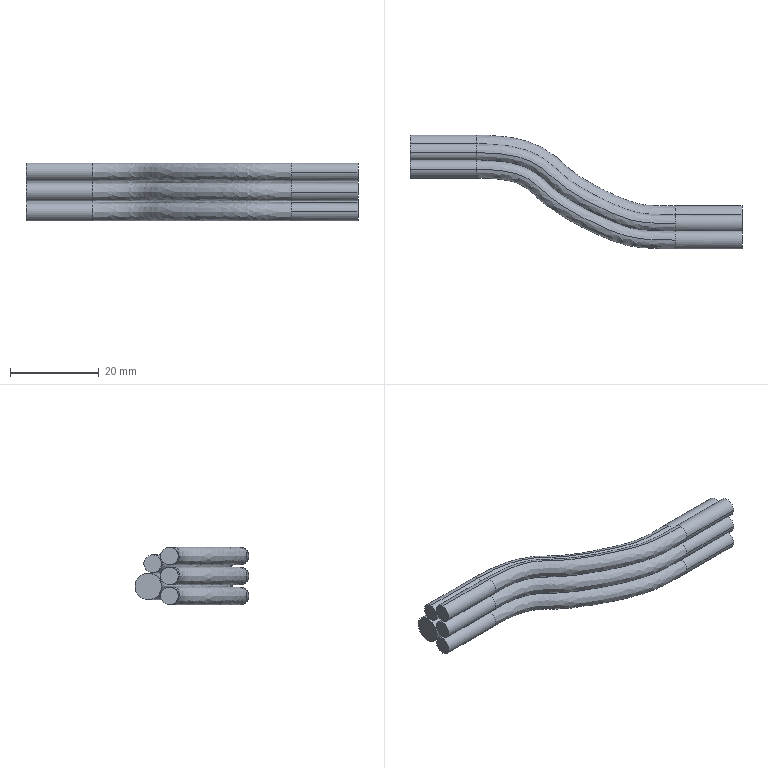Part | STEP file | 5 solids | 40 faces | box 75 x 25.743 x 13 mm | volume 6214 mm3 | cylinder 20 | plane 10 | spline 10 | commonest cylinder face diameters 4 x16 6 x4